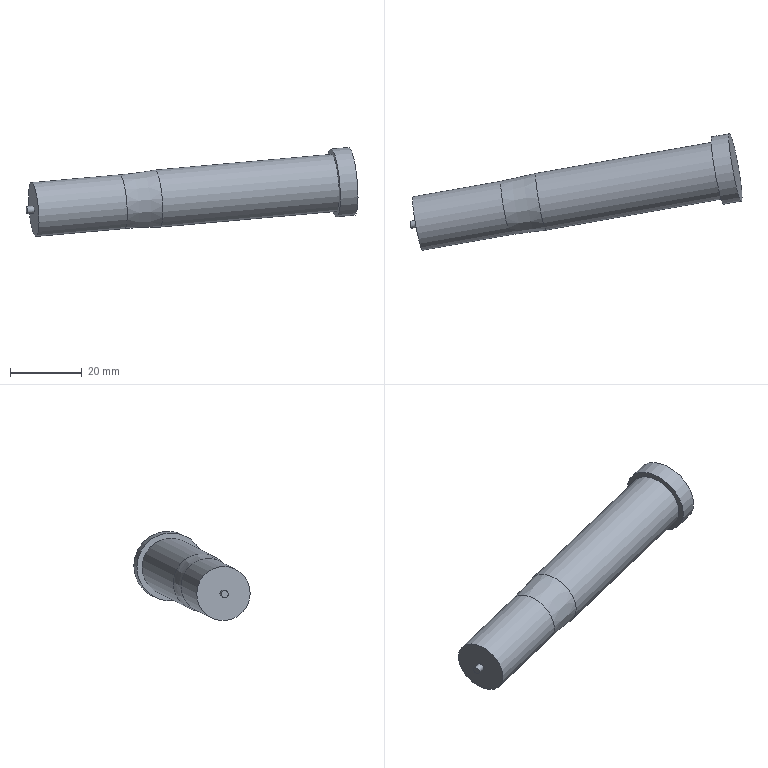Part | NX | features solid 2 | 1 solid | 9 faces | box 92.291 x 32.362 x 24.829 mm | volume 17854 mm3 | plane 4 | cylinder 4 | cone 1 | commonest cylinder face diameters 2 x1 15.1 x1 16 x1 19 x1
STEP:
#1=CARTESIAN_POINT('',(-582.127,-32.436,30.583));
#2=VERTEX_POINT('',#1);
#3=CARTESIAN_POINT('',(-582.301,-31.451,30.583));
#4=DIRECTION('',(-0.9811,-0.173,-0.08716));
#5=DIRECTION('',(0.1736,-0.9848,0.));
#6=AXIS2_PLACEMENT_3D('',#3,#4,#5);
#7=CIRCLE('',#6,1.);
#8=EDGE_CURVE('',#2,#2,#7,.T.);
#9=ORIENTED_EDGE('',*,*,#8,.F.);
#10=EDGE_LOOP('',(#9));
#11=FACE_BOUND('',#10,.T.);
#12=CARTESIAN_POINT('',(-583.612,-24.016,30.583));
#13=VERTEX_POINT('',#12);
#14=CARTESIAN_POINT('',(-582.301,-31.451,30.583));
#15=DIRECTION('',(0.9811,0.173,0.08716));
#16=DIRECTION('',(-0.1736,0.9848,0.));
#17=AXIS2_PLACEMENT_3D('',#14,#15,#16);
#18=CIRCLE('',#17,7.55);
#19=EDGE_CURVE('',#13,#13,#18,.T.);
#20=ORIENTED_EDGE('',*,*,#19,.F.);
#21=EDGE_LOOP('',(#20));
#22=FACE_BOUND('',#21,.T.);
#23=CARTESIAN_POINT('',(-582.301,-31.451,30.583));
#24=DIRECTION('',(-0.9811,-0.173,-0.08716));
#25=DIRECTION('',(0.1736,-0.9848,0.));
#26=AXIS2_PLACEMENT_3D('',#23,#24,#25);
#27=PLANE('',#26);
#28=ADVANCED_FACE('',(#11,#22),#27,.T.);
#29=CARTESIAN_POINT('',(-559.086,-19.691,32.762));
#30=VERTEX_POINT('',#29);
#31=CARTESIAN_POINT('',(-557.775,-27.126,32.762));
#32=DIRECTION('',(0.9811,0.173,0.08716));
#33=DIRECTION('',(-0.1736,0.9848,0.));
#34=AXIS2_PLACEMENT_3D('',#31,#32,#33);
#35=CIRCLE('',#34,7.55);
#36=EDGE_CURVE('',#30,#30,#35,.T.);
#37=ORIENTED_EDGE('',*,*,#36,.F.);
#38=EDGE_LOOP('',(#37));
#39=FACE_BOUND('',#38,.T.);
#40=ORIENTED_EDGE('',*,*,#19,.T.);
#41=EDGE_LOOP('',(#40));
#42=FACE_BOUND('',#41,.T.);
#43=CARTESIAN_POINT('',(-582.301,-31.451,30.583));
#44=DIRECTION('',(0.9811,0.173,0.08716));
#45=DIRECTION('',(-0.1736,0.9848,0.));
#46=AXIS2_PLACEMENT_3D('',#43,#44,#45);
#47=CYLINDRICAL_SURFACE('',#46,7.55);
#48=ADVANCED_FACE('',(#39,#42),#47,.T.);
#49=ORIENTED_EDGE('',*,*,#36,.T.);
#50=EDGE_LOOP('',(#49));
#51=FACE_BOUND('',#50,.T.);
#52=CARTESIAN_POINT('',(-549.353,-17.518,33.633));
#53=VERTEX_POINT('',#52);
#54=CARTESIAN_POINT('',(-547.964,-25.396,33.633));
#55=DIRECTION('',(0.9811,0.173,0.08716));
#56=DIRECTION('',(-0.1736,0.9848,0.));
#57=AXIS2_PLACEMENT_3D('',#54,#55,#56);
#58=CIRCLE('',#57,8.);
#59=EDGE_CURVE('',#53,#53,#58,.T.);
#60=ORIENTED_EDGE('',*,*,#59,.F.);
#61=EDGE_LOOP('',(#60));
#62=FACE_BOUND('',#61,.T.);
#63=CARTESIAN_POINT('',(-557.775,-27.126,32.762));
#64=DIRECTION('',(0.9811,0.173,0.08716));
#65=DIRECTION('',(-0.1736,0.9848,0.));
#66=AXIS2_PLACEMENT_3D('',#63,#64,#65);
#67=CONICAL_SURFACE('',#66,7.55,0.04497);
#68=ADVANCED_FACE('',(#51,#62),#67,.T.);
#69=CARTESIAN_POINT('',(-497.522,-24.626,37.991));
#70=VERTEX_POINT('',#69);
#71=CARTESIAN_POINT('',(-498.911,-16.747,37.991));
#72=DIRECTION('',(-0.9811,-0.173,-0.08716));
#73=DIRECTION('',(0.1736,-0.9848,0.));
#74=AXIS2_PLACEMENT_3D('',#71,#72,#73);
#75=CIRCLE('',#74,8.);
#76=EDGE_CURVE('',#70,#70,#75,.F.);
#77=ORIENTED_EDGE('',*,*,#76,.F.);
#78=EDGE_LOOP('',(#77));
#79=FACE_BOUND('',#78,.T.);
#80=ORIENTED_EDGE('',*,*,#59,.T.);
#81=EDGE_LOOP('',(#80));
#82=FACE_BOUND('',#81,.T.);
#83=CARTESIAN_POINT('',(-547.964,-25.396,33.633));
#84=DIRECTION('',(0.9811,0.173,0.08716));
#85=DIRECTION('',(-0.1736,0.9848,0.));
#86=AXIS2_PLACEMENT_3D('',#83,#84,#85);
#87=CYLINDRICAL_SURFACE('',#86,8.);
#88=ADVANCED_FACE('',(#79,#82),#87,.T.);
#89=CARTESIAN_POINT('',(-492.356,-25.238,38.427));
#90=VERTEX_POINT('',#89);
#91=CARTESIAN_POINT('',(-494.006,-15.882,38.427));
#92=DIRECTION('',(-0.9811,-0.173,-0.08716));
#93=DIRECTION('',(0.1736,-0.9848,0.));
#94=AXIS2_PLACEMENT_3D('',#91,#92,#93);
#95=CIRCLE('',#94,9.5);
#96=EDGE_CURVE('',#90,#90,#95,.T.);
#97=ORIENTED_EDGE('',*,*,#96,.F.);
#98=EDGE_LOOP('',(#97));
#99=FACE_BOUND('',#98,.T.);
#100=CARTESIAN_POINT('',(-494.006,-15.882,38.427));
#101=DIRECTION('',(0.9811,0.173,0.08716));
#102=DIRECTION('',(-0.1736,0.9848,0.));
#103=AXIS2_PLACEMENT_3D('',#100,#101,#102);
#104=PLANE('',#103);
#105=ADVANCED_FACE('',(#99),#104,.T.);
#106=ORIENTED_EDGE('',*,*,#76,.T.);
#107=EDGE_LOOP('',(#106));
#108=FACE_BOUND('',#107,.T.);
#109=CARTESIAN_POINT('',(-500.561,-7.391,37.991));
#110=VERTEX_POINT('',#109);
#111=CARTESIAN_POINT('',(-498.911,-16.747,37.991));
#112=DIRECTION('',(0.9811,0.173,0.08716));
#113=DIRECTION('',(-0.1736,0.9848,0.));
#114=AXIS2_PLACEMENT_3D('',#111,#112,#113);
#115=CIRCLE('',#114,9.5);
#116=EDGE_CURVE('',#110,#110,#115,.T.);
#117=ORIENTED_EDGE('',*,*,#116,.F.);
#118=EDGE_LOOP('',(#117));
#119=FACE_BOUND('',#118,.T.);
#120=CARTESIAN_POINT('',(-498.911,-16.747,37.991));
#121=DIRECTION('',(-0.9811,-0.173,-0.08716));
#122=DIRECTION('',(0.1736,-0.9848,0.));
#123=AXIS2_PLACEMENT_3D('',#120,#121,#122);
#124=PLANE('',#123);
#125=ADVANCED_FACE('',(#108,#119),#124,.T.);
#126=ORIENTED_EDGE('',*,*,#96,.T.);
#127=EDGE_LOOP('',(#126));
#128=FACE_BOUND('',#127,.T.);
#129=ORIENTED_EDGE('',*,*,#116,.T.);
#130=EDGE_LOOP('',(#129));
#131=FACE_BOUND('',#130,.T.);
#132=CARTESIAN_POINT('',(-498.911,-16.747,37.991));
#133=DIRECTION('',(0.9811,0.173,0.08716));
#134=DIRECTION('',(-0.1736,0.9848,0.));
#135=AXIS2_PLACEMENT_3D('',#132,#133,#134);
#136=CYLINDRICAL_SURFACE('',#135,9.5);
#137=ADVANCED_FACE('',(#128,#131),#136,.T.);
#138=CARTESIAN_POINT('',(-584.437,-30.812,30.408));
#139=VERTEX_POINT('',#138);
#140=CARTESIAN_POINT('',(-584.263,-31.797,30.408));
#141=DIRECTION('',(0.9811,0.173,0.08716));
#142=DIRECTION('',(-0.1736,0.9848,0.));
#143=AXIS2_PLACEMENT_3D('',#140,#141,#142);
#144=CIRCLE('',#143,1.);
#145=EDGE_CURVE('',#139,#139,#144,.T.);
#146=ORIENTED_EDGE('',*,*,#145,.F.);
#147=EDGE_LOOP('',(#146));
#148=FACE_BOUND('',#147,.T.);
#149=CARTESIAN_POINT('',(-584.263,-31.797,30.408));
#150=DIRECTION('',(-0.9811,-0.173,-0.08716));
#151=DIRECTION('',(0.1736,-0.9848,0.));
#152=AXIS2_PLACEMENT_3D('',#149,#150,#151);
#153=PLANE('',#152);
#154=ADVANCED_FACE('',(#148),#153,.T.);
#155=ORIENTED_EDGE('',*,*,#145,.T.);
#156=EDGE_LOOP('',(#155));
#157=FACE_BOUND('',#156,.T.);
#158=ORIENTED_EDGE('',*,*,#8,.T.);
#159=EDGE_LOOP('',(#158));
#160=FACE_BOUND('',#159,.T.);
#161=CARTESIAN_POINT('',(-582.301,-31.451,30.583));
#162=DIRECTION('',(-0.9811,-0.173,-0.08716));
#163=DIRECTION('',(0.1736,-0.9848,0.));
#164=AXIS2_PLACEMENT_3D('',#161,#162,#163);
#165=CYLINDRICAL_SURFACE('',#164,1.);
#166=ADVANCED_FACE('',(#157,#160),#165,.T.);
#167=CLOSED_SHELL('',(#28,#48,#68,#88,#105,#125,#137,#154,#166));
#168=MANIFOLD_SOLID_BREP('',#167);
#169=(LENGTH_UNIT()NAMED_UNIT(*)SI_UNIT(.MILLI.,.METRE.));
#170=UNCERTAINTY_MEASURE_WITH_UNIT(LENGTH_MEASURE(0.00001),#169,'','');
#171=(NAMED_UNIT(*)PLANE_ANGLE_UNIT()SI_UNIT($,.RADIAN.));
#172=(NAMED_UNIT(*)SI_UNIT($,.STERADIAN.)SOLID_ANGLE_UNIT());
#173=(GEOMETRIC_REPRESENTATION_CONTEXT(3)GLOBAL_UNCERTAINTY_ASSIGNED_CONTEXT((#170))GLOBAL_UNIT_ASSIGNED_CONTEXT((#169,#171,#172))REPRESENTATION_CONTEXT('',''));
#174=ADVANCED_BREP_SHAPE_REPRESENTATION('',(#168),#173);